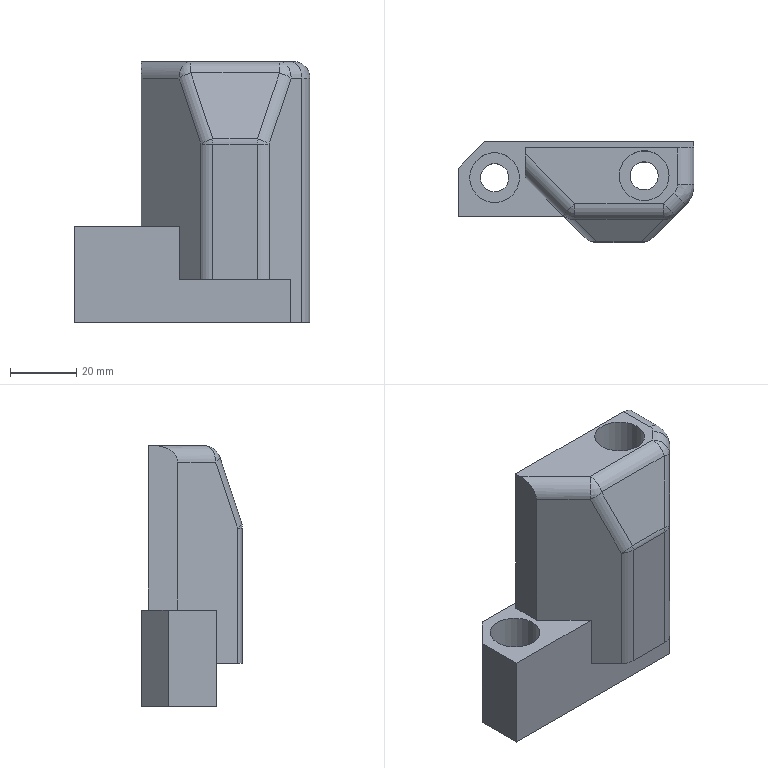Part | STEP file | gslz 2016.10.28-13_id310_x_t | 1 solid | 42 faces | box 71 x 30.372 x 78.5 mm | volume 87139 mm3 | plane 21 | cylinder 16 | sphere 4 | spline 1 | commonest cylinder face diameters 10 x11 8.5 x2 15 x2 17 x1